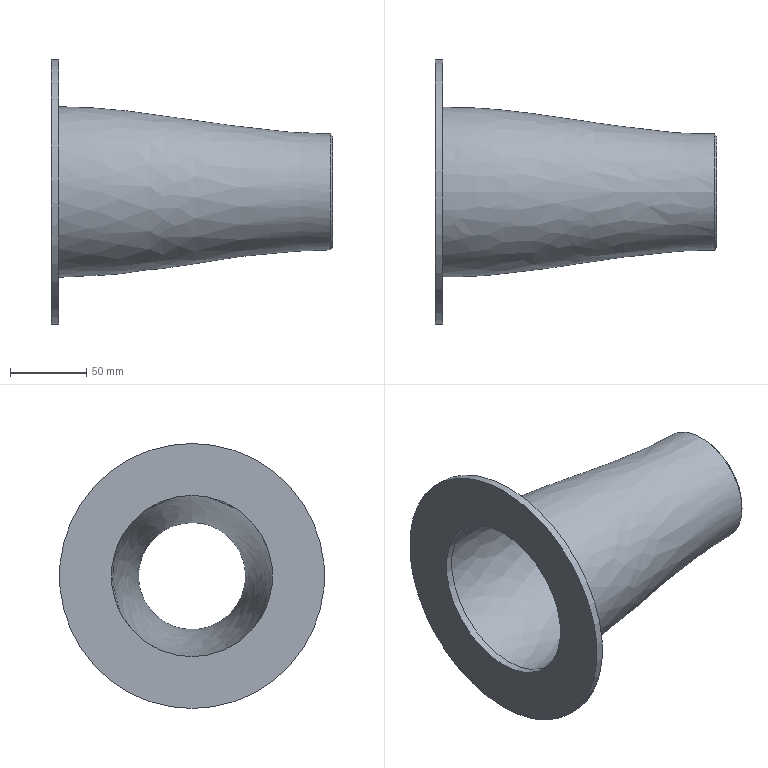Part | STEP file | Reducer Secondary | 1 solid | 8 faces | box 185 x 174 x 174 mm | volume 229980 mm3 | spline 3 | plane 3 | cylinder 2 | commonest cylinder face diameters 106 x1 174 x1
STEP:
#1=CARTESIAN_POINT('',(-39.141,-5.989,-10.37));
#2=VERTEX_POINT('',#1);
#3=CARTESIAN_POINT('',(-39.2,-5.989,-10.311));
#4=VERTEX_POINT('',#3);
#5=CARTESIAN_POINT('',(-39.141,-5.989,-10.37));
#6=DIRECTION('',(-0.7062,0.,0.708));
#7=VECTOR('',#6,0.3937);
#8=LINE('',#5,#7);
#9=EDGE_CURVE('',#2,#4,#8,.T.);
#10=ORIENTED_EDGE('',*,*,#9,.T.);
#11=CARTESIAN_POINT('',(-39.2,-5.989,-10.311));
#12=CARTESIAN_POINT('',(-39.2,-6.213,-10.311));
#13=CARTESIAN_POINT('',(-39.2,-6.662,-10.413));
#14=CARTESIAN_POINT('',(-39.2,-7.202,-10.844));
#15=CARTESIAN_POINT('',(-39.2,-7.501,-11.466));
#16=CARTESIAN_POINT('',(-39.2,-7.501,-12.079));
#17=CARTESIAN_POINT('',(-39.2,-7.308,-12.572));
#18=CARTESIAN_POINT('',(-39.2,-7.025,-12.927));
#19=CARTESIAN_POINT('',(-39.2,-6.712,-13.14));
#20=CARTESIAN_POINT('',(-39.2,-6.433,-13.25));
#21=CARTESIAN_POINT('',(-39.2,-6.14,-13.317));
#22=CARTESIAN_POINT('',(-39.2,-5.762,-13.317));
#23=CARTESIAN_POINT('',(-39.2,-5.328,-13.183));
#24=CARTESIAN_POINT('',(-39.2,-4.953,-12.927));
#25=CARTESIAN_POINT('',(-39.2,-4.67,-12.572));
#26=CARTESIAN_POINT('',(-39.2,-4.505,-12.15));
#27=CARTESIAN_POINT('',(-39.2,-4.458,-11.546));
#28=CARTESIAN_POINT('',(-39.2,-4.715,-10.891));
#29=CARTESIAN_POINT('',(-39.2,-5.316,-10.413));
#30=CARTESIAN_POINT('',(-39.2,-5.765,-10.311));
#31=CARTESIAN_POINT('',(-39.2,-5.989,-10.311));
#32=B_SPLINE_CURVE_WITH_KNOTS('',3,(#11,#12,#13,#14,#15,#16,#17,#18,#19,#20,#21,#22,#23,#24,#25,#26,#27,#28,#29,#30,#31),.UNSPECIFIED.,.T.,.F.,(4,1,1,1,1,1,1,1,1,1,1,1,1,1,1,1,1,1,4),(-3.142,-2.693,-2.244,-1.795,-1.346,-1.047,-0.748,-0.4488,-0.2992,-0.1496,0.1496,0.4488,0.748,1.047,1.346,1.646,2.244,2.693,3.142),.UNSPECIFIED.);
#33=EDGE_CURVE('',#4,#4,#32,.T.);
#34=ORIENTED_EDGE('',*,*,#33,.T.);
#35=ORIENTED_EDGE('',*,*,#9,.F.);
#36=CARTESIAN_POINT('',(-39.141,-5.989,-10.37));
#37=CARTESIAN_POINT('',(-39.141,-5.773,-10.37));
#38=CARTESIAN_POINT('',(-39.141,-5.343,-10.469));
#39=CARTESIAN_POINT('',(-39.141,-4.765,-10.928));
#40=CARTESIAN_POINT('',(-39.141,-4.519,-11.556));
#41=CARTESIAN_POINT('',(-39.141,-4.563,-12.137));
#42=CARTESIAN_POINT('',(-39.141,-4.722,-12.542));
#43=CARTESIAN_POINT('',(-39.141,-4.994,-12.883));
#44=CARTESIAN_POINT('',(-39.141,-5.354,-13.129));
#45=CARTESIAN_POINT('',(-39.141,-5.771,-13.257));
#46=CARTESIAN_POINT('',(-39.141,-6.134,-13.257));
#47=CARTESIAN_POINT('',(-39.141,-6.415,-13.193));
#48=CARTESIAN_POINT('',(-39.141,-6.684,-13.088));
#49=CARTESIAN_POINT('',(-39.141,-6.984,-12.883));
#50=CARTESIAN_POINT('',(-39.141,-7.256,-12.542));
#51=CARTESIAN_POINT('',(-39.141,-7.442,-12.069));
#52=CARTESIAN_POINT('',(-39.141,-7.442,-11.479));
#53=CARTESIAN_POINT('',(-39.141,-7.154,-10.882));
#54=CARTESIAN_POINT('',(-39.141,-6.635,-10.468));
#55=CARTESIAN_POINT('',(-39.141,-6.204,-10.37));
#56=CARTESIAN_POINT('',(-39.141,-5.989,-10.37));
#57=B_SPLINE_CURVE_WITH_KNOTS('',3,(#36,#37,#38,#39,#40,#41,#42,#43,#44,#45,#46,#47,#48,#49,#50,#51,#52,#53,#54,#55,#56),.UNSPECIFIED.,.T.,.F.,(4,1,1,1,1,1,1,1,1,1,1,1,1,1,1,1,1,1,4),(-3.142,-2.693,-2.244,-1.646,-1.346,-1.047,-0.748,-0.4488,-0.1496,0.1496,0.2992,0.4488,0.748,1.047,1.346,1.795,2.244,2.693,3.142),.UNSPECIFIED.);
#58=EDGE_CURVE('',#2,#2,#57,.T.);
#59=ORIENTED_EDGE('',*,*,#58,.T.);
#60=EDGE_LOOP('',(#10,#34,#35,#59));
#61=FACE_OUTER_BOUND('',#60,.T.);
#62=CARTESIAN_POINT('',(-39.141,-5.989,-10.37));
#63=CARTESIAN_POINT('',(-39.141,-6.204,-10.37));
#64=CARTESIAN_POINT('',(-39.141,-6.635,-10.468));
#65=CARTESIAN_POINT('',(-39.141,-7.154,-10.882));
#66=CARTESIAN_POINT('',(-39.141,-7.442,-11.479));
#67=CARTESIAN_POINT('',(-39.141,-7.442,-12.069));
#68=CARTESIAN_POINT('',(-39.141,-7.256,-12.542));
#69=CARTESIAN_POINT('',(-39.141,-6.984,-12.883));
#70=CARTESIAN_POINT('',(-39.141,-6.684,-13.088));
#71=CARTESIAN_POINT('',(-39.141,-6.415,-13.193));
#72=CARTESIAN_POINT('',(-39.141,-6.134,-13.257));
#73=CARTESIAN_POINT('',(-39.141,-5.771,-13.257));
#74=CARTESIAN_POINT('',(-39.141,-5.354,-13.129));
#75=CARTESIAN_POINT('',(-39.141,-4.994,-12.883));
#76=CARTESIAN_POINT('',(-39.141,-4.722,-12.542));
#77=CARTESIAN_POINT('',(-39.141,-4.563,-12.137));
#78=CARTESIAN_POINT('',(-39.141,-4.519,-11.556));
#79=CARTESIAN_POINT('',(-39.141,-4.765,-10.928));
#80=CARTESIAN_POINT('',(-39.141,-5.343,-10.469));
#81=CARTESIAN_POINT('',(-39.141,-5.773,-10.37));
#82=CARTESIAN_POINT('',(-39.141,-5.989,-10.37));
#83=CARTESIAN_POINT('',(-39.161,-5.989,-10.35));
#84=CARTESIAN_POINT('',(-39.161,-6.207,-10.35));
#85=CARTESIAN_POINT('',(-39.161,-6.644,-10.45));
#86=CARTESIAN_POINT('',(-39.161,-7.17,-10.869));
#87=CARTESIAN_POINT('',(-39.161,-7.462,-11.475));
#88=CARTESIAN_POINT('',(-39.161,-7.462,-12.072));
#89=CARTESIAN_POINT('',(-39.161,-7.273,-12.552));
#90=CARTESIAN_POINT('',(-39.161,-6.997,-12.898));
#91=CARTESIAN_POINT('',(-39.161,-6.693,-13.105));
#92=CARTESIAN_POINT('',(-39.161,-6.421,-13.212));
#93=CARTESIAN_POINT('',(-39.161,-6.136,-13.277));
#94=CARTESIAN_POINT('',(-39.161,-5.768,-13.277));
#95=CARTESIAN_POINT('',(-39.161,-5.346,-13.147));
#96=CARTESIAN_POINT('',(-39.161,-4.981,-12.898));
#97=CARTESIAN_POINT('',(-39.161,-4.705,-12.552));
#98=CARTESIAN_POINT('',(-39.161,-4.544,-12.141));
#99=CARTESIAN_POINT('',(-39.161,-4.498,-11.553));
#100=CARTESIAN_POINT('',(-39.161,-4.749,-10.916));
#101=CARTESIAN_POINT('',(-39.161,-5.334,-10.45));
#102=CARTESIAN_POINT('',(-39.161,-5.77,-10.35));
#103=CARTESIAN_POINT('',(-39.161,-5.989,-10.35));
#104=CARTESIAN_POINT('',(-39.18,-5.989,-10.331));
#105=CARTESIAN_POINT('',(-39.18,-6.21,-10.331));
#106=CARTESIAN_POINT('',(-39.18,-6.653,-10.432));
#107=CARTESIAN_POINT('',(-39.18,-7.186,-10.856));
#108=CARTESIAN_POINT('',(-39.18,-7.482,-11.47));
#109=CARTESIAN_POINT('',(-39.18,-7.482,-12.076));
#110=CARTESIAN_POINT('',(-39.18,-7.29,-12.562));
#111=CARTESIAN_POINT('',(-39.18,-7.011,-12.913));
#112=CARTESIAN_POINT('',(-39.18,-6.703,-13.123));
#113=CARTESIAN_POINT('',(-39.18,-6.427,-13.231));
#114=CARTESIAN_POINT('',(-39.18,-6.138,-13.297));
#115=CARTESIAN_POINT('',(-39.18,-5.765,-13.297));
#116=CARTESIAN_POINT('',(-39.18,-5.337,-13.165));
#117=CARTESIAN_POINT('',(-39.18,-4.967,-12.913));
#118=CARTESIAN_POINT('',(-39.18,-4.687,-12.562));
#119=CARTESIAN_POINT('',(-39.18,-4.524,-12.145));
#120=CARTESIAN_POINT('',(-39.18,-4.478,-11.549));
#121=CARTESIAN_POINT('',(-39.18,-4.732,-10.903));
#122=CARTESIAN_POINT('',(-39.18,-5.325,-10.432));
#123=CARTESIAN_POINT('',(-39.18,-5.767,-10.331));
#124=CARTESIAN_POINT('',(-39.18,-5.989,-10.331));
#125=CARTESIAN_POINT('',(-39.2,-5.989,-10.311));
#126=CARTESIAN_POINT('',(-39.2,-6.213,-10.311));
#127=CARTESIAN_POINT('',(-39.2,-6.662,-10.413));
#128=CARTESIAN_POINT('',(-39.2,-7.202,-10.844));
#129=CARTESIAN_POINT('',(-39.2,-7.501,-11.466));
#130=CARTESIAN_POINT('',(-39.2,-7.501,-12.079));
#131=CARTESIAN_POINT('',(-39.2,-7.308,-12.572));
#132=CARTESIAN_POINT('',(-39.2,-7.025,-12.927));
#133=CARTESIAN_POINT('',(-39.2,-6.712,-13.14));
#134=CARTESIAN_POINT('',(-39.2,-6.433,-13.25));
#135=CARTESIAN_POINT('',(-39.2,-6.14,-13.317));
#136=CARTESIAN_POINT('',(-39.2,-5.762,-13.317));
#137=CARTESIAN_POINT('',(-39.2,-5.328,-13.183));
#138=CARTESIAN_POINT('',(-39.2,-4.953,-12.927));
#139=CARTESIAN_POINT('',(-39.2,-4.67,-12.572));
#140=CARTESIAN_POINT('',(-39.2,-4.505,-12.15));
#141=CARTESIAN_POINT('',(-39.2,-4.458,-11.546));
#142=CARTESIAN_POINT('',(-39.2,-4.715,-10.891));
#143=CARTESIAN_POINT('',(-39.2,-5.316,-10.413));
#144=CARTESIAN_POINT('',(-39.2,-5.765,-10.311));
#145=CARTESIAN_POINT('',(-39.2,-5.989,-10.311));
#146=B_SPLINE_SURFACE_WITH_KNOTS('',3,3,((#62,#63,#64,#65,#66,#67,#68,#69,#70,#71,#72,#73,#74,#75,#76,#77,#78,#79,#80,#81,#82),(#83,#84,#85,#86,#87,#88,#89,#90,#91,#92,#93,#94,#95,#96,#97,#98,#99,#100,#101,#102,#103),(#104,#105,#106,#107,#108,#109,#110,#111,#112,#113,#114,#115,#116,#117,#118,#119,#120,#121,#122,#123,#124),(#125,#126,#127,#128,#129,#130,#131,#132,#133,#134,#135,#136,#137,#138,#139,#140,#141,#142,#143,#144,#145)),.UNSPECIFIED.,.F.,.T.,.F.,(4,4),(4,1,1,1,1,1,1,1,1,1,1,1,1,1,1,1,1,1,4),(0.,1.),(-3.142,-2.693,-2.244,-1.795,-1.346,-1.047,-0.748,-0.4488,-0.2992,-0.1496,0.1496,0.4488,0.748,1.047,1.346,1.646,2.244,2.693,3.142),.UNSPECIFIED.);
#147=ADVANCED_FACE('',(#61),#146,.T.);
#148=ORIENTED_EDGE('',*,*,#33,.F.);
#149=CARTESIAN_POINT('',(-46.227,-5.989,-9.606));
#150=VERTEX_POINT('',#149);
#151=CARTESIAN_POINT('',(-39.2,-5.989,-10.311));
#152=CARTESIAN_POINT('',(-41.542,-5.989,-10.299));
#153=CARTESIAN_POINT('',(-43.885,-5.989,-9.606));
#154=CARTESIAN_POINT('',(-46.227,-5.989,-9.606));
#155=B_SPLINE_CURVE_WITH_KNOTS('',3,(#151,#152,#153,#154),.UNSPECIFIED.,.F.,.F.,(4,4),(0.008333,1.),.UNSPECIFIED.);
#156=EDGE_CURVE('',#4,#150,#155,.T.);
#157=ORIENTED_EDGE('',*,*,#156,.T.);
#158=CARTESIAN_POINT('',(-46.227,-5.989,-11.811));
#159=DIRECTION('',(1.,0.,0.));
#160=DIRECTION('',(0.,0.,-1.));
#161=AXIS2_PLACEMENT_3D('',#158,#159,#160);
#162=CIRCLE('',#161,2.205);
#163=EDGE_CURVE('',#150,#150,#162,.T.);
#164=ORIENTED_EDGE('',*,*,#163,.T.);
#165=ORIENTED_EDGE('',*,*,#156,.F.);
#166=EDGE_LOOP('',(#148,#157,#164,#165));
#167=FACE_OUTER_BOUND('',#166,.T.);
#168=CARTESIAN_POINT('',(-39.2,-5.989,-10.311));
#169=CARTESIAN_POINT('',(-41.542,-5.989,-10.299));
#170=CARTESIAN_POINT('',(-43.885,-5.989,-9.606));
#171=CARTESIAN_POINT('',(-46.227,-5.989,-9.606));
#172=CARTESIAN_POINT('',(-39.2,-6.213,-10.311));
#173=CARTESIAN_POINT('',(-41.542,-6.215,-10.299));
#174=CARTESIAN_POINT('',(-43.885,-6.319,-9.606));
#175=CARTESIAN_POINT('',(-46.227,-6.319,-9.606));
#176=CARTESIAN_POINT('',(-39.2,-6.662,-10.413));
#177=CARTESIAN_POINT('',(-41.542,-6.667,-10.402));
#178=CARTESIAN_POINT('',(-43.885,-6.978,-9.757));
#179=CARTESIAN_POINT('',(-46.227,-6.978,-9.757));
#180=CARTESIAN_POINT('',(-39.2,-7.142,-10.796));
#181=CARTESIAN_POINT('',(-41.542,-7.151,-10.788));
#182=CARTESIAN_POINT('',(-43.885,-7.683,-10.319));
#183=CARTESIAN_POINT('',(-46.227,-7.683,-10.319));
#184=CARTESIAN_POINT('',(-39.2,-7.406,-11.255));
#185=CARTESIAN_POINT('',(-41.542,-7.417,-11.251));
#186=CARTESIAN_POINT('',(-43.885,-8.072,-10.994));
#187=CARTESIAN_POINT('',(-46.227,-8.072,-10.994));
#188=CARTESIAN_POINT('',(-39.2,-7.507,-11.697));
#189=CARTESIAN_POINT('',(-41.542,-7.519,-11.696));
#190=CARTESIAN_POINT('',(-43.885,-8.221,-11.644));
#191=CARTESIAN_POINT('',(-46.227,-8.221,-11.644));
#192=CARTESIAN_POINT('',(-39.2,-7.473,-12.15));
#193=CARTESIAN_POINT('',(-41.542,-7.485,-12.153));
#194=CARTESIAN_POINT('',(-43.885,-8.171,-12.309));
#195=CARTESIAN_POINT('',(-46.227,-8.171,-12.309));
#196=CARTESIAN_POINT('',(-39.2,-7.308,-12.572));
#197=CARTESIAN_POINT('',(-41.542,-7.318,-12.578));
#198=CARTESIAN_POINT('',(-43.885,-7.927,-12.93));
#199=CARTESIAN_POINT('',(-46.227,-7.927,-12.93));
#200=CARTESIAN_POINT('',(-39.2,-7.025,-12.927));
#201=CARTESIAN_POINT('',(-41.542,-7.033,-12.936));
#202=CARTESIAN_POINT('',(-43.885,-7.511,-13.452));
#203=CARTESIAN_POINT('',(-46.227,-7.511,-13.452));
#204=CARTESIAN_POINT('',(-39.2,-6.65,-13.183));
#205=CARTESIAN_POINT('',(-41.542,-6.655,-13.194));
#206=CARTESIAN_POINT('',(-43.885,-6.96,-13.827));
#207=CARTESIAN_POINT('',(-46.227,-6.96,-13.827));
#208=CARTESIAN_POINT('',(-39.2,-6.216,-13.317));
#209=CARTESIAN_POINT('',(-41.542,-6.218,-13.328));
#210=CARTESIAN_POINT('',(-43.885,-6.322,-14.024));
#211=CARTESIAN_POINT('',(-46.227,-6.322,-14.024));
#212=CARTESIAN_POINT('',(-39.2,-5.762,-13.317));
#213=CARTESIAN_POINT('',(-41.542,-5.76,-13.328));
#214=CARTESIAN_POINT('',(-43.885,-5.655,-14.024));
#215=CARTESIAN_POINT('',(-46.227,-5.655,-14.024));
#216=CARTESIAN_POINT('',(-39.2,-5.328,-13.183));
#217=CARTESIAN_POINT('',(-41.542,-5.323,-13.194));
#218=CARTESIAN_POINT('',(-43.885,-5.018,-13.827));
#219=CARTESIAN_POINT('',(-46.227,-5.018,-13.827));
#220=CARTESIAN_POINT('',(-39.2,-4.953,-12.927));
#221=CARTESIAN_POINT('',(-41.542,-4.945,-12.936));
#222=CARTESIAN_POINT('',(-43.885,-4.467,-13.452));
#223=CARTESIAN_POINT('',(-46.227,-4.467,-13.452));
#224=CARTESIAN_POINT('',(-39.2,-4.67,-12.572));
#225=CARTESIAN_POINT('',(-41.542,-4.66,-12.578));
#226=CARTESIAN_POINT('',(-43.885,-4.051,-12.93));
#227=CARTESIAN_POINT('',(-46.227,-4.051,-12.93));
#228=CARTESIAN_POINT('',(-39.2,-4.477,-12.079));
#229=CARTESIAN_POINT('',(-41.542,-4.465,-12.082));
#230=CARTESIAN_POINT('',(-43.885,-3.766,-12.206));
#231=CARTESIAN_POINT('',(-46.227,-3.766,-12.206));
#232=CARTESIAN_POINT('',(-39.2,-4.476,-11.466));
#233=CARTESIAN_POINT('',(-41.542,-4.465,-11.463));
#234=CARTESIAN_POINT('',(-43.885,-3.766,-11.304));
#235=CARTESIAN_POINT('',(-46.227,-3.766,-11.304));
#236=CARTESIAN_POINT('',(-39.2,-4.776,-10.844));
#237=CARTESIAN_POINT('',(-41.542,-4.767,-10.836));
#238=CARTESIAN_POINT('',(-43.885,-4.206,-10.389));
#239=CARTESIAN_POINT('',(-46.227,-4.206,-10.389));
#240=CARTESIAN_POINT('',(-39.2,-5.316,-10.413));
#241=CARTESIAN_POINT('',(-41.542,-5.311,-10.403));
#242=CARTESIAN_POINT('',(-43.885,-5.,-9.757));
#243=CARTESIAN_POINT('',(-46.227,-5.,-9.757));
#244=CARTESIAN_POINT('',(-39.2,-5.765,-10.311));
#245=CARTESIAN_POINT('',(-41.542,-5.763,-10.299));
#246=CARTESIAN_POINT('',(-43.885,-5.659,-9.606));
#247=CARTESIAN_POINT('',(-46.227,-5.659,-9.606));
#248=CARTESIAN_POINT('',(-39.2,-5.989,-10.311));
#249=CARTESIAN_POINT('',(-41.542,-5.989,-10.299));
#250=CARTESIAN_POINT('',(-43.885,-5.989,-9.606));
#251=CARTESIAN_POINT('',(-46.227,-5.989,-9.606));
#252=B_SPLINE_SURFACE_WITH_KNOTS('',3,3,((#168,#169,#170,#171),(#172,#173,#174,#175),(#176,#177,#178,#179),(#180,#181,#182,#183),(#184,#185,#186,#187),(#188,#189,#190,#191),(#192,#193,#194,#195),(#196,#197,#198,#199),(#200,#201,#202,#203),(#204,#205,#206,#207),(#208,#209,#210,#211),(#212,#213,#214,#215),(#216,#217,#218,#219),(#220,#221,#222,#223),(#224,#225,#226,#227),(#228,#229,#230,#231),(#232,#233,#234,#235),(#236,#237,#238,#239),(#240,#241,#242,#243),(#244,#245,#246,#247),(#248,#249,#250,#251)),.UNSPECIFIED.,.T.,.F.,.F.,(4,1,1,1,1,1,1,1,1,1,1,1,1,1,1,1,1,1,4),(4,4),(0.,0.07143,0.1429,0.1905,0.2381,0.2857,0.3333,0.381,0.4286,0.4762,0.5238,0.5714,0.619,0.6667,0.7143,0.7857,0.8571,0.9286,1.),(0.008333,1.),.UNSPECIFIED.);
#253=ADVANCED_FACE('',(#167),#252,.F.);
#254=ORIENTED_EDGE('',*,*,#58,.F.);
#255=EDGE_LOOP('',(#254));
#256=FACE_OUTER_BOUND('',#255,.T.);
#257=CARTESIAN_POINT('',(-39.141,-5.989,-10.429));
#258=VERTEX_POINT('',#257);
#259=CARTESIAN_POINT('',(-39.141,-5.989,-10.429));
#260=CARTESIAN_POINT('',(-39.141,-5.782,-10.429));
#261=CARTESIAN_POINT('',(-39.141,-5.369,-10.523));
#262=CARTESIAN_POINT('',(-39.141,-4.872,-10.92));
#263=CARTESIAN_POINT('',(-39.141,-4.596,-11.493));
#264=CARTESIAN_POINT('',(-39.141,-4.596,-12.058));
#265=CARTESIAN_POINT('',(-39.141,-4.774,-12.512));
#266=CARTESIAN_POINT('',(-39.141,-5.035,-12.839));
#267=CARTESIAN_POINT('',(-39.141,-5.38,-13.075));
#268=CARTESIAN_POINT('',(-39.141,-5.78,-13.198));
#269=CARTESIAN_POINT('',(-39.141,-6.198,-13.198));
#270=CARTESIAN_POINT('',(-39.141,-6.598,-13.075));
#271=CARTESIAN_POINT('',(-39.141,-6.943,-12.839));
#272=CARTESIAN_POINT('',(-39.141,-7.204,-12.512));
#273=CARTESIAN_POINT('',(-39.141,-7.356,-12.123));
#274=CARTESIAN_POINT('',(-39.141,-7.388,-11.706));
#275=CARTESIAN_POINT('',(-39.141,-7.295,-11.299));
#276=CARTESIAN_POINT('',(-39.141,-7.051,-10.876));
#277=CARTESIAN_POINT('',(-39.141,-6.609,-10.523));
#278=CARTESIAN_POINT('',(-39.141,-6.196,-10.429));
#279=CARTESIAN_POINT('',(-39.141,-5.989,-10.429));
#280=B_SPLINE_CURVE_WITH_KNOTS('',3,(#259,#260,#261,#262,#263,#264,#265,#266,#267,#268,#269,#270,#271,#272,#273,#274,#275,#276,#277,#278,#279),.UNSPECIFIED.,.T.,.F.,(4,1,1,1,1,1,1,1,1,1,1,1,1,1,1,1,1,1,4),(-1.,-0.9286,-0.8571,-0.7857,-0.7143,-0.6667,-0.619,-0.5714,-0.5238,-0.4762,-0.4286,-0.381,-0.3333,-0.2857,-0.2381,-0.1905,-0.1429,-0.07143,0.),.UNSPECIFIED.);
#281=EDGE_CURVE('',#258,#258,#280,.T.);
#282=ORIENTED_EDGE('',*,*,#281,.T.);
#283=EDGE_LOOP('',(#282));
#284=FACE_BOUND('',#283,.T.);
#285=CARTESIAN_POINT('',(-39.141,-5.989,-11.811));
#286=DIRECTION('',(1.,0.,0.));
#287=DIRECTION('',(0.,0.,-1.));
#288=AXIS2_PLACEMENT_3D('',#285,#286,#287);
#289=PLANE('',#288);
#290=ADVANCED_FACE('',(#256,#284),#289,.T.);
#291=CARTESIAN_POINT('',(-46.227,-5.989,-15.236));
#292=VERTEX_POINT('',#291);
#293=CARTESIAN_POINT('',(-46.227,-5.989,-11.811));
#294=DIRECTION('',(1.,0.,0.));
#295=DIRECTION('',(0.,0.,1.));
#296=AXIS2_PLACEMENT_3D('',#293,#294,#295);
#297=CIRCLE('',#296,3.425);
#298=EDGE_CURVE('',#292,#292,#297,.T.);
#299=ORIENTED_EDGE('',*,*,#298,.F.);
#300=CARTESIAN_POINT('',(-46.424,-5.989,-15.236));
#301=VERTEX_POINT('',#300);
#302=CARTESIAN_POINT('',(-46.424,-5.989,-15.236));
#303=DIRECTION('',(-1.,0.,0.));
#304=VECTOR('',#303,3.425);
#305=LINE('',#302,#304);
#306=EDGE_CURVE('',#292,#301,#305,.T.);
#307=ORIENTED_EDGE('',*,*,#306,.T.);
#308=CARTESIAN_POINT('',(-46.424,-5.989,-11.811));
#309=DIRECTION('',(-1.,0.,0.));
#310=DIRECTION('',(0.,0.,1.));
#311=AXIS2_PLACEMENT_3D('',#308,#309,#310);
#312=CIRCLE('',#311,3.425);
#313=EDGE_CURVE('',#301,#301,#312,.T.);
#314=ORIENTED_EDGE('',*,*,#313,.F.);
#315=ORIENTED_EDGE('',*,*,#306,.F.);
#316=EDGE_LOOP('',(#299,#307,#314,#315));
#317=FACE_OUTER_BOUND('',#316,.T.);
#318=CARTESIAN_POINT('',(-46.424,-5.989,-11.811));
#319=DIRECTION('',(1.,0.,0.));
#320=DIRECTION('',(0.,0.,1.));
#321=AXIS2_PLACEMENT_3D('',#318,#319,#320);
#322=CYLINDRICAL_SURFACE('',#321,3.425);
#323=ADVANCED_FACE('',(#317),#322,.T.);
#324=ORIENTED_EDGE('',*,*,#298,.T.);
#325=EDGE_LOOP('',(#324));
#326=FACE_OUTER_BOUND('',#325,.T.);
#327=ORIENTED_EDGE('',*,*,#163,.F.);
#328=EDGE_LOOP('',(#327));
#329=FACE_BOUND('',#328,.T.);
#330=CARTESIAN_POINT('',(-46.227,-5.989,-11.811));
#331=DIRECTION('',(-1.,0.,0.));
#332=DIRECTION('',(0.,0.,1.));
#333=AXIS2_PLACEMENT_3D('',#330,#331,#332);
#334=PLANE('',#333);
#335=ADVANCED_FACE('',(#326,#329),#334,.F.);
#336=CARTESIAN_POINT('',(-46.227,-5.989,-9.724));
#337=VERTEX_POINT('',#336);
#338=CARTESIAN_POINT('',(-46.227,-5.989,-13.898));
#339=VERTEX_POINT('',#338);
#340=CARTESIAN_POINT('',(-46.227,-5.989,-11.811));
#341=DIRECTION('',(1.,0.,0.));
#342=DIRECTION('',(0.,0.,-1.));
#343=AXIS2_PLACEMENT_3D('',#340,#341,#342);
#344=CIRCLE('',#343,2.087);
#345=EDGE_CURVE('',#337,#339,#344,.T.);
#346=ORIENTED_EDGE('',*,*,#345,.T.);
#347=CARTESIAN_POINT('',(-46.424,-5.989,-13.898));
#348=VERTEX_POINT('',#347);
#349=CARTESIAN_POINT('',(-46.227,-5.989,-13.898));
#350=DIRECTION('',(-1.,0.,0.));
#351=VECTOR('',#350,2.205);
#352=LINE('',#349,#351);
#353=EDGE_CURVE('',#339,#348,#352,.T.);
#354=ORIENTED_EDGE('',*,*,#353,.T.);
#355=CARTESIAN_POINT('',(-46.424,-5.989,-11.811));
#356=DIRECTION('',(1.,0.,0.));
#357=DIRECTION('',(0.,0.,1.));
#358=AXIS2_PLACEMENT_3D('',#355,#356,#357);
#359=CIRCLE('',#358,2.087);
#360=EDGE_CURVE('',#348,#348,#359,.T.);
#361=ORIENTED_EDGE('',*,*,#360,.F.);
#362=ORIENTED_EDGE('',*,*,#353,.F.);
#363=CARTESIAN_POINT('',(-46.227,-5.989,-11.811));
#364=DIRECTION('',(1.,0.,0.));
#365=DIRECTION('',(0.,0.,-1.));
#366=AXIS2_PLACEMENT_3D('',#363,#364,#365);
#367=CIRCLE('',#366,2.087);
#368=EDGE_CURVE('',#339,#337,#367,.T.);
#369=ORIENTED_EDGE('',*,*,#368,.T.);
#370=EDGE_LOOP('',(#346,#354,#361,#362,#369));
#371=FACE_OUTER_BOUND('',#370,.T.);
#372=CARTESIAN_POINT('',(-46.227,-5.989,-11.811));
#373=DIRECTION('',(-1.,0.,0.));
#374=DIRECTION('',(0.,0.,1.));
#375=AXIS2_PLACEMENT_3D('',#372,#373,#374);
#376=CYLINDRICAL_SURFACE('',#375,2.087);
#377=ADVANCED_FACE('',(#371),#376,.F.);
#378=ORIENTED_EDGE('',*,*,#281,.F.);
#379=CARTESIAN_POINT('',(-39.141,-5.989,-10.429));
#380=CARTESIAN_POINT('',(-40.504,-5.989,-10.429));
#381=CARTESIAN_POINT('',(-42.876,-5.989,-10.024));
#382=CARTESIAN_POINT('',(-45.225,-5.989,-9.724));
#383=CARTESIAN_POINT('',(-46.227,-5.989,-9.724));
#384=B_SPLINE_CURVE_WITH_KNOTS('',3,(#379,#380,#381,#382,#383),.UNSPECIFIED.,.F.,.F.,(4,1,4),(0.,0.5714,1.),.UNSPECIFIED.);
#385=EDGE_CURVE('',#258,#337,#384,.T.);
#386=ORIENTED_EDGE('',*,*,#385,.T.);
#387=ORIENTED_EDGE('',*,*,#368,.F.);
#388=ORIENTED_EDGE('',*,*,#345,.F.);
#389=ORIENTED_EDGE('',*,*,#385,.F.);
#390=EDGE_LOOP('',(#378,#386,#387,#388,#389));
#391=FACE_OUTER_BOUND('',#390,.T.);
#392=CARTESIAN_POINT('',(-39.141,-5.989,-10.429));
#393=CARTESIAN_POINT('',(-40.504,-5.989,-10.429));
#394=CARTESIAN_POINT('',(-42.876,-5.989,-10.024));
#395=CARTESIAN_POINT('',(-45.225,-5.989,-9.724));
#396=CARTESIAN_POINT('',(-46.227,-5.989,-9.724));
#397=CARTESIAN_POINT('',(-39.141,-6.196,-10.429));
#398=CARTESIAN_POINT('',(-40.504,-6.196,-10.429));
#399=CARTESIAN_POINT('',(-42.876,-6.256,-10.024));
#400=CARTESIAN_POINT('',(-45.225,-6.301,-9.724));
#401=CARTESIAN_POINT('',(-46.227,-6.301,-9.724));
#402=CARTESIAN_POINT('',(-39.141,-6.609,-10.523));
#403=CARTESIAN_POINT('',(-40.504,-6.609,-10.523));
#404=CARTESIAN_POINT('',(-42.876,-6.791,-10.146));
#405=CARTESIAN_POINT('',(-45.225,-6.925,-9.867));
#406=CARTESIAN_POINT('',(-46.227,-6.925,-9.867));
#407=CARTESIAN_POINT('',(-39.141,-7.051,-10.876));
#408=CARTESIAN_POINT('',(-40.504,-7.051,-10.876));
#409=CARTESIAN_POINT('',(-42.876,-7.362,-10.602));
#410=CARTESIAN_POINT('',(-45.225,-7.593,-10.399));
#411=CARTESIAN_POINT('',(-46.227,-7.593,-10.399));
#412=CARTESIAN_POINT('',(-39.141,-7.295,-11.299));
#413=CARTESIAN_POINT('',(-40.504,-7.295,-11.299));
#414=CARTESIAN_POINT('',(-42.876,-7.677,-11.148));
#415=CARTESIAN_POINT('',(-45.225,-7.96,-11.037));
#416=CARTESIAN_POINT('',(-46.227,-7.96,-11.037));
#417=CARTESIAN_POINT('',(-39.141,-7.388,-11.706));
#418=CARTESIAN_POINT('',(-40.504,-7.388,-11.706));
#419=CARTESIAN_POINT('',(-42.876,-7.798,-11.675));
#420=CARTESIAN_POINT('',(-45.225,-8.101,-11.653));
#421=CARTESIAN_POINT('',(-46.227,-8.101,-11.653));
#422=CARTESIAN_POINT('',(-39.141,-7.356,-12.123));
#423=CARTESIAN_POINT('',(-40.504,-7.356,-12.123));
#424=CARTESIAN_POINT('',(-42.876,-7.757,-12.215));
#425=CARTESIAN_POINT('',(-45.225,-8.054,-12.282));
#426=CARTESIAN_POINT('',(-46.227,-8.054,-12.282));
#427=CARTESIAN_POINT('',(-39.141,-7.204,-12.512));
#428=CARTESIAN_POINT('',(-40.504,-7.204,-12.512));
#429=CARTESIAN_POINT('',(-42.876,-7.56,-12.718));
#430=CARTESIAN_POINT('',(-45.225,-7.823,-12.87));
#431=CARTESIAN_POINT('',(-46.227,-7.823,-12.87));
#432=CARTESIAN_POINT('',(-39.141,-6.943,-12.839));
#433=CARTESIAN_POINT('',(-40.504,-6.943,-12.839));
#434=CARTESIAN_POINT('',(-42.876,-7.223,-13.141));
#435=CARTESIAN_POINT('',(-45.225,-7.429,-13.364));
#436=CARTESIAN_POINT('',(-46.227,-7.429,-13.364));
#437=CARTESIAN_POINT('',(-39.141,-6.598,-13.075));
#438=CARTESIAN_POINT('',(-40.504,-6.598,-13.075));
#439=CARTESIAN_POINT('',(-42.876,-6.776,-13.445));
#440=CARTESIAN_POINT('',(-45.225,-6.908,-13.719));
#441=CARTESIAN_POINT('',(-46.227,-6.908,-13.719));
#442=CARTESIAN_POINT('',(-39.141,-6.198,-13.198));
#443=CARTESIAN_POINT('',(-40.504,-6.198,-13.198));
#444=CARTESIAN_POINT('',(-42.876,-6.259,-13.605));
#445=CARTESIAN_POINT('',(-45.225,-6.305,-13.905));
#446=CARTESIAN_POINT('',(-46.227,-6.305,-13.905));
#447=CARTESIAN_POINT('',(-39.141,-5.78,-13.198));
#448=CARTESIAN_POINT('',(-40.504,-5.78,-13.198));
#449=CARTESIAN_POINT('',(-42.876,-5.719,-13.605));
#450=CARTESIAN_POINT('',(-45.225,-5.673,-13.905));
#451=CARTESIAN_POINT('',(-46.227,-5.673,-13.905));
#452=CARTESIAN_POINT('',(-39.141,-5.38,-13.075));
#453=CARTESIAN_POINT('',(-40.504,-5.38,-13.075));
#454=CARTESIAN_POINT('',(-42.876,-5.202,-13.445));
#455=CARTESIAN_POINT('',(-45.225,-5.07,-13.719));
#456=CARTESIAN_POINT('',(-46.227,-5.07,-13.719));
#457=CARTESIAN_POINT('',(-39.141,-5.035,-12.839));
#458=CARTESIAN_POINT('',(-40.504,-5.035,-12.839));
#459=CARTESIAN_POINT('',(-42.876,-4.755,-13.141));
#460=CARTESIAN_POINT('',(-45.225,-4.548,-13.364));
#461=CARTESIAN_POINT('',(-46.227,-4.548,-13.364));
#462=CARTESIAN_POINT('',(-39.141,-4.774,-12.512));
#463=CARTESIAN_POINT('',(-40.504,-4.774,-12.512));
#464=CARTESIAN_POINT('',(-42.876,-4.418,-12.718));
#465=CARTESIAN_POINT('',(-45.225,-4.155,-12.87));
#466=CARTESIAN_POINT('',(-46.227,-4.155,-12.87));
#467=CARTESIAN_POINT('',(-39.141,-4.596,-12.058));
#468=CARTESIAN_POINT('',(-40.504,-4.596,-12.058));
#469=CARTESIAN_POINT('',(-42.876,-4.187,-12.131));
#470=CARTESIAN_POINT('',(-45.225,-3.885,-12.184));
#471=CARTESIAN_POINT('',(-46.227,-3.885,-12.184));
#472=CARTESIAN_POINT('',(-39.141,-4.596,-11.493));
#473=CARTESIAN_POINT('',(-40.504,-4.596,-11.493));
#474=CARTESIAN_POINT('',(-42.876,-4.187,-11.4));
#475=CARTESIAN_POINT('',(-45.225,-3.885,-11.331));
#476=CARTESIAN_POINT('',(-46.227,-3.885,-11.331));
#477=CARTESIAN_POINT('',(-39.141,-4.872,-10.92));
#478=CARTESIAN_POINT('',(-40.504,-4.872,-10.92));
#479=CARTESIAN_POINT('',(-42.876,-4.544,-10.659));
#480=CARTESIAN_POINT('',(-45.225,-4.302,-10.466));
#481=CARTESIAN_POINT('',(-46.227,-4.302,-10.466));
#482=CARTESIAN_POINT('',(-39.141,-5.369,-10.523));
#483=CARTESIAN_POINT('',(-40.504,-5.369,-10.523));
#484=CARTESIAN_POINT('',(-42.876,-5.187,-10.146));
#485=CARTESIAN_POINT('',(-45.225,-5.053,-9.867));
#486=CARTESIAN_POINT('',(-46.227,-5.053,-9.867));
#487=CARTESIAN_POINT('',(-39.141,-5.782,-10.429));
#488=CARTESIAN_POINT('',(-40.504,-5.782,-10.429));
#489=CARTESIAN_POINT('',(-42.876,-5.722,-10.024));
#490=CARTESIAN_POINT('',(-45.225,-5.677,-9.724));
#491=CARTESIAN_POINT('',(-46.227,-5.677,-9.724));
#492=CARTESIAN_POINT('',(-39.141,-5.989,-10.429));
#493=CARTESIAN_POINT('',(-40.504,-5.989,-10.429));
#494=CARTESIAN_POINT('',(-42.876,-5.989,-10.024));
#495=CARTESIAN_POINT('',(-45.225,-5.989,-9.724));
#496=CARTESIAN_POINT('',(-46.227,-5.989,-9.724));
#497=B_SPLINE_SURFACE_WITH_KNOTS('',3,3,((#392,#393,#394,#395,#396),(#397,#398,#399,#400,#401),(#402,#403,#404,#405,#406),(#407,#408,#409,#410,#411),(#412,#413,#414,#415,#416),(#417,#418,#419,#420,#421),(#422,#423,#424,#425,#426),(#427,#428,#429,#430,#431),(#432,#433,#434,#435,#436),(#437,#438,#439,#440,#441),(#442,#443,#444,#445,#446),(#447,#448,#449,#450,#451),(#452,#453,#454,#455,#456),(#457,#458,#459,#460,#461),(#462,#463,#464,#465,#466),(#467,#468,#469,#470,#471),(#472,#473,#474,#475,#476),(#477,#478,#479,#480,#481),(#482,#483,#484,#485,#486),(#487,#488,#489,#490,#491),(#492,#493,#494,#495,#496)),.UNSPECIFIED.,.T.,.F.,.F.,(4,1,1,1,1,1,1,1,1,1,1,1,1,1,1,1,1,1,4),(4,1,4),(0.,0.07143,0.1429,0.1905,0.2381,0.2857,0.3333,0.381,0.4286,0.4762,0.5238,0.5714,0.619,0.6667,0.7143,0.7857,0.8571,0.9286,1.),(0.,0.5714,1.),.UNSPECIFIED.);
#498=ADVANCED_FACE('',(#391),#497,.T.);
#499=ORIENTED_EDGE('',*,*,#313,.T.);
#500=EDGE_LOOP('',(#499));
#501=FACE_OUTER_BOUND('',#500,.T.);
#502=ORIENTED_EDGE('',*,*,#360,.T.);
#503=EDGE_LOOP('',(#502));
#504=FACE_BOUND('',#503,.T.);
#505=CARTESIAN_POINT('',(-46.424,-5.989,-11.811));
#506=DIRECTION('',(-1.,0.,0.));
#507=DIRECTION('',(0.,0.,1.));
#508=AXIS2_PLACEMENT_3D('',#505,#506,#507);
#509=PLANE('',#508);
#510=ADVANCED_FACE('',(#501,#504),#509,.T.);
#511=CLOSED_SHELL('',(#147,#253,#290,#323,#335,#377,#498,#510));
#512=MANIFOLD_SOLID_BREP('',#511);
#513=(LENGTH_UNIT()NAMED_UNIT(*)SI_UNIT(.MILLI.,.METRE.));
#514=LENGTH_MEASURE_WITH_UNIT(LENGTH_MEASURE(25.4),#513);
#515=DIMENSIONAL_EXPONENTS(1.,0.,0.,0.,0.,0.,0.);
#516=(CONVERSION_BASED_UNIT('inch',#514)LENGTH_UNIT()NAMED_UNIT(#515));
#517=UNCERTAINTY_MEASURE_WITH_UNIT(LENGTH_MEASURE(0.0003937),#516,'','');
#518=(NAMED_UNIT(*)PLANE_ANGLE_UNIT()SI_UNIT($,.RADIAN.));
#519=(NAMED_UNIT(*)SI_UNIT($,.STERADIAN.)SOLID_ANGLE_UNIT());
#520=(GEOMETRIC_REPRESENTATION_CONTEXT(3)GLOBAL_UNCERTAINTY_ASSIGNED_CONTEXT((#517))GLOBAL_UNIT_ASSIGNED_CONTEXT((#516,#518,#519))REPRESENTATION_CONTEXT('',''));
#521=ADVANCED_BREP_SHAPE_REPRESENTATION('',(#512),#520);